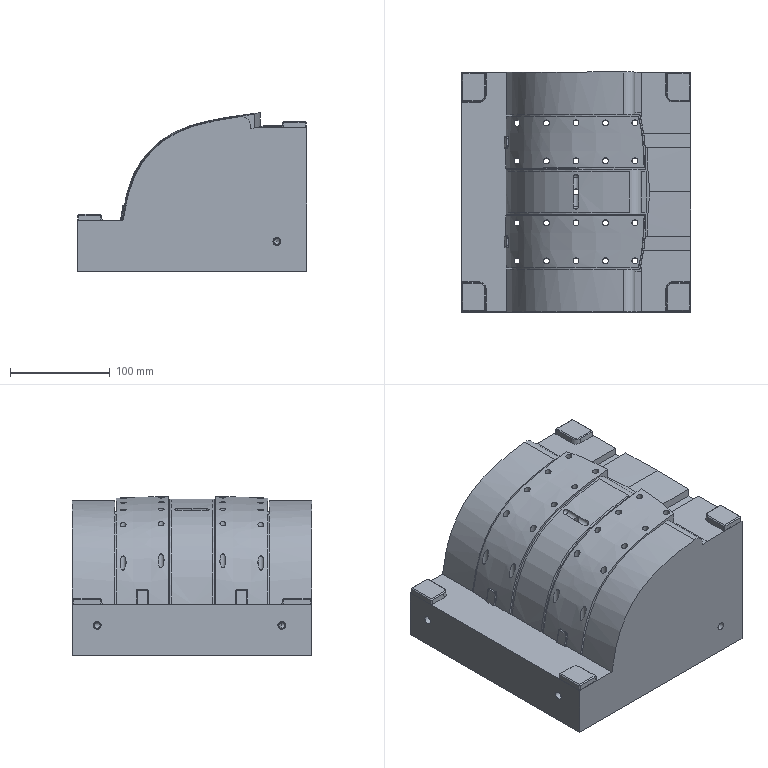Part | NX | features solid 2 | 1 solid | 260 faces | box 230 x 240 x 159.014 mm | volume 6548136 mm3 | spline 101 | plane 87 | cylinder 60 | cone 10 | sphere 2 | commonest cylinder face diameters 6 x36 2 x12 8 x5 13 x4 20 x3